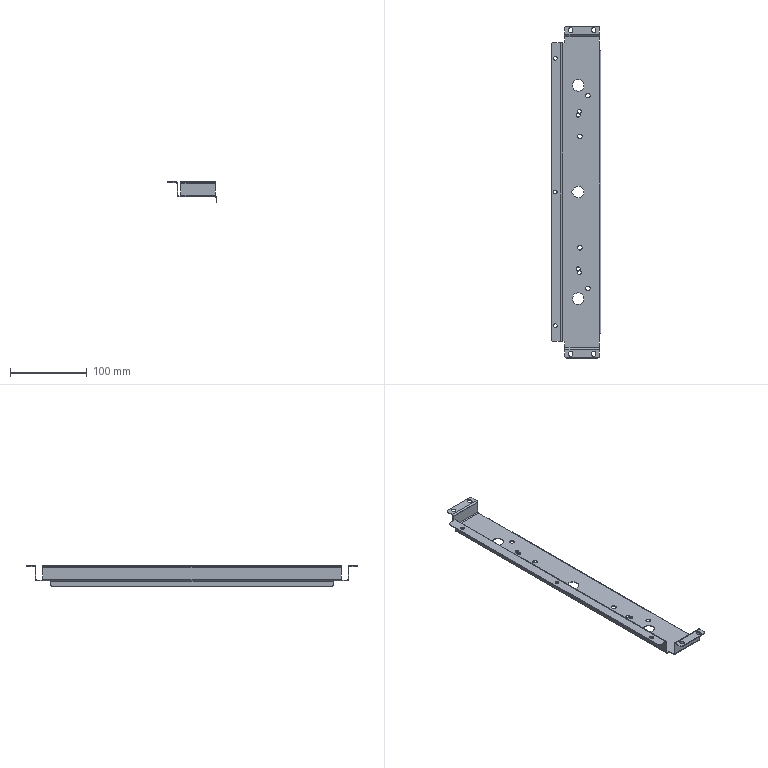Part | SolidWorks | features BaseBody 1 | 1 solid | 127 faces | box 65 x 432 x 26.6 mm | volume 36858 mm3 | cylinder 65 | plane 62 | commonest cylinder face diameters 5 x28 4 x15 2 x9 6 x8 15 x5